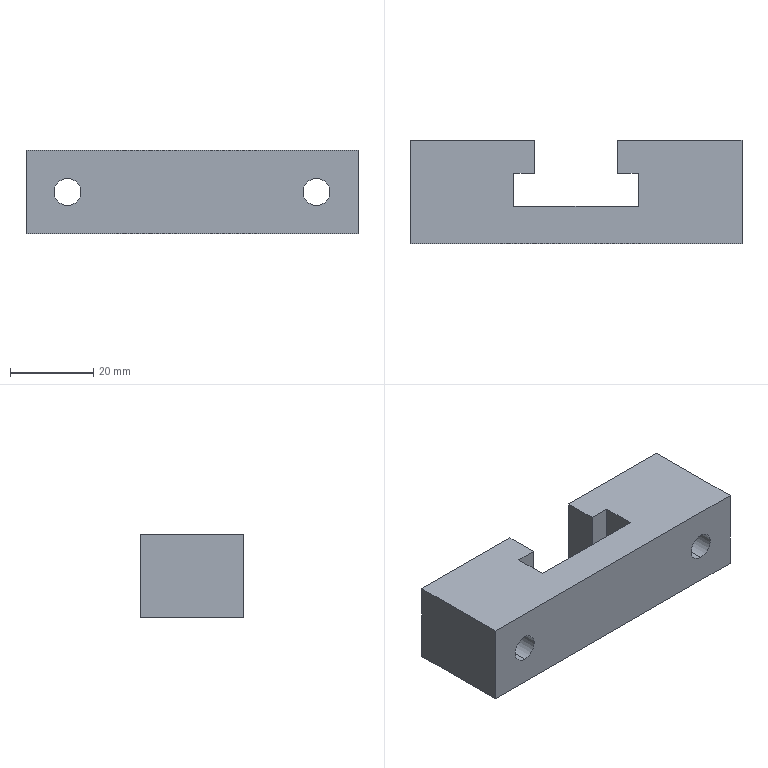Part | STEP file | A14-026 | 1 solid | 24 faces | box 80 x 25 x 20 mm | volume 29104 mm3 | plane 16 | cylinder 8 | commonest cylinder face diameters 6.5 x4 11 x4